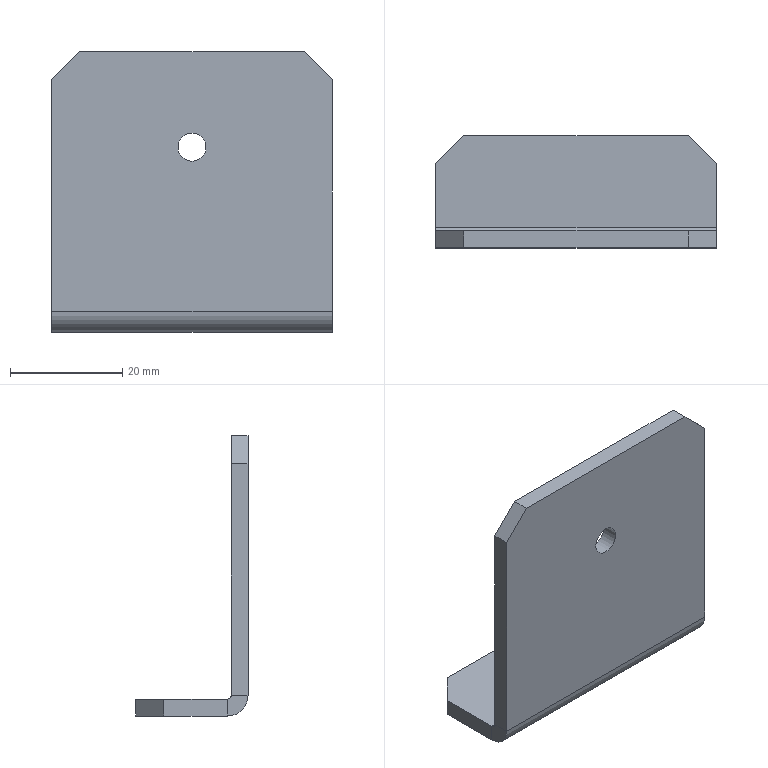Part | NX | 1 solid | 19 faces | box 50 x 20 x 50 mm | volume 9696 mm3 | plane 16 | cylinder 3 | commonest cylinder face diameters 1.5 x1 5 x1 7.5 x1
STEP:
#1=CARTESIAN_POINT('',(25.,0.,3.75));
#2=VERTEX_POINT('',#1);
#3=CARTESIAN_POINT('',(25.,3.,3.75));
#4=VERTEX_POINT('',#3);
#5=CARTESIAN_POINT('',(25.,0.,3.75));
#6=DIRECTION('',(0.,1.,0.));
#7=VECTOR('',#6,1000.);
#8=LINE('',#5,#7);
#9=EDGE_CURVE('',#2,#4,#8,.T.);
#10=ORIENTED_EDGE('',*,*,#9,.F.);
#11=CARTESIAN_POINT('',(25.,3.75,0.));
#12=VERTEX_POINT('',#11);
#13=CARTESIAN_POINT('',(25.,3.75,3.75));
#14=DIRECTION('',(1.,0.,0.));
#15=DIRECTION('',(0.,0.,-1.));
#16=AXIS2_PLACEMENT_3D('',#13,#14,#15);
#17=CIRCLE('',#16,3.75);
#18=EDGE_CURVE('',#12,#2,#17,.F.);
#19=ORIENTED_EDGE('',*,*,#18,.F.);
#20=CARTESIAN_POINT('',(25.,3.75,3.));
#21=VERTEX_POINT('',#20);
#22=CARTESIAN_POINT('',(25.,3.75,3.));
#23=DIRECTION('',(0.,0.,-1.));
#24=VECTOR('',#23,1000.);
#25=LINE('',#22,#24);
#26=EDGE_CURVE('',#21,#12,#25,.T.);
#27=ORIENTED_EDGE('',*,*,#26,.F.);
#28=CARTESIAN_POINT('',(25.,3.75,3.75));
#29=DIRECTION('',(1.,0.,0.));
#30=DIRECTION('',(0.,0.,-1.));
#31=AXIS2_PLACEMENT_3D('',#28,#29,#30);
#32=CIRCLE('',#31,0.75);
#33=EDGE_CURVE('',#21,#4,#32,.F.);
#34=ORIENTED_EDGE('',*,*,#33,.T.);
#35=EDGE_LOOP('',(#10,#19,#27,#34));
#36=FACE_BOUND('',#35,.T.);
#37=CARTESIAN_POINT('',(25.,0.,3.75));
#38=DIRECTION('',(1.,0.,0.));
#39=DIRECTION('',(0.,0.,-1.));
#40=AXIS2_PLACEMENT_3D('',#37,#38,#39);
#41=PLANE('',#40);
#42=ADVANCED_FACE('',(#36),#41,.T.);
#43=CARTESIAN_POINT('',(25.,3.,45.));
#44=VERTEX_POINT('',#43);
#45=CARTESIAN_POINT('',(25.,3.,0.));
#46=DIRECTION('',(0.,0.,1.));
#47=VECTOR('',#46,1000.);
#48=LINE('',#45,#47);
#49=EDGE_CURVE('',#4,#44,#48,.T.);
#50=ORIENTED_EDGE('',*,*,#49,.T.);
#51=CARTESIAN_POINT('',(25.,0.,45.));
#52=VERTEX_POINT('',#51);
#53=CARTESIAN_POINT('',(25.,3.75,45.));
#54=DIRECTION('',(0.,-1.,0.));
#55=VECTOR('',#54,1000.);
#56=LINE('',#53,#55);
#57=EDGE_CURVE('',#44,#52,#56,.T.);
#58=ORIENTED_EDGE('',*,*,#57,.T.);
#59=CARTESIAN_POINT('',(25.,0.,0.));
#60=DIRECTION('',(0.,0.,1.));
#61=VECTOR('',#60,1000.);
#62=LINE('',#59,#61);
#63=EDGE_CURVE('',#2,#52,#62,.T.);
#64=ORIENTED_EDGE('',*,*,#63,.F.);
#65=ORIENTED_EDGE('',*,*,#9,.T.);
#66=EDGE_LOOP('',(#50,#58,#64,#65));
#67=FACE_BOUND('',#66,.T.);
#68=CARTESIAN_POINT('',(25.,3.75,3.));
#69=DIRECTION('',(1.,0.,0.));
#70=DIRECTION('',(0.,0.,-1.));
#71=AXIS2_PLACEMENT_3D('',#68,#69,#70);
#72=PLANE('',#71);
#73=ADVANCED_FACE('',(#67),#72,.T.);
#74=CARTESIAN_POINT('',(-25.,3.75,0.));
#75=VERTEX_POINT('',#74);
#76=CARTESIAN_POINT('',(-25.,3.75,3.));
#77=VERTEX_POINT('',#76);
#78=CARTESIAN_POINT('',(-25.,3.75,0.));
#79=DIRECTION('',(0.,0.,1.));
#80=VECTOR('',#79,1000.);
#81=LINE('',#78,#80);
#82=EDGE_CURVE('',#75,#77,#81,.T.);
#83=ORIENTED_EDGE('',*,*,#82,.F.);
#84=CARTESIAN_POINT('',(-25.,0.,3.75));
#85=VERTEX_POINT('',#84);
#86=CARTESIAN_POINT('',(-25.,3.75,3.75));
#87=DIRECTION('',(1.,0.,0.));
#88=DIRECTION('',(0.,0.,-1.));
#89=AXIS2_PLACEMENT_3D('',#86,#87,#88);
#90=CIRCLE('',#89,3.75);
#91=EDGE_CURVE('',#75,#85,#90,.F.);
#92=ORIENTED_EDGE('',*,*,#91,.T.);
#93=CARTESIAN_POINT('',(-25.,3.,3.75));
#94=VERTEX_POINT('',#93);
#95=CARTESIAN_POINT('',(-25.,3.,3.75));
#96=DIRECTION('',(0.,-1.,0.));
#97=VECTOR('',#96,1000.);
#98=LINE('',#95,#97);
#99=EDGE_CURVE('',#94,#85,#98,.T.);
#100=ORIENTED_EDGE('',*,*,#99,.F.);
#101=CARTESIAN_POINT('',(-25.,3.75,3.75));
#102=DIRECTION('',(1.,0.,0.));
#103=DIRECTION('',(0.,0.,-1.));
#104=AXIS2_PLACEMENT_3D('',#101,#102,#103);
#105=CIRCLE('',#104,0.75);
#106=EDGE_CURVE('',#77,#94,#105,.F.);
#107=ORIENTED_EDGE('',*,*,#106,.F.);
#108=EDGE_LOOP('',(#83,#92,#100,#107));
#109=FACE_BOUND('',#108,.T.);
#110=CARTESIAN_POINT('',(-25.,3.75,0.));
#111=DIRECTION('',(-1.,0.,0.));
#112=DIRECTION('',(0.,0.,1.));
#113=AXIS2_PLACEMENT_3D('',#110,#111,#112);
#114=PLANE('',#113);
#115=ADVANCED_FACE('',(#109),#114,.T.);
#116=CARTESIAN_POINT('',(-25.,15.,3.));
#117=VERTEX_POINT('',#116);
#118=CARTESIAN_POINT('',(-25.,20.,3.));
#119=DIRECTION('',(0.,-1.,0.));
#120=VECTOR('',#119,1000.);
#121=LINE('',#118,#120);
#122=EDGE_CURVE('',#117,#77,#121,.T.);
#123=ORIENTED_EDGE('',*,*,#122,.F.);
#124=CARTESIAN_POINT('',(-25.,15.,0.));
#125=VERTEX_POINT('',#124);
#126=CARTESIAN_POINT('',(-25.,15.,3.75));
#127=DIRECTION('',(0.,0.,-1.));
#128=VECTOR('',#127,1000.);
#129=LINE('',#126,#128);
#130=EDGE_CURVE('',#117,#125,#129,.T.);
#131=ORIENTED_EDGE('',*,*,#130,.T.);
#132=CARTESIAN_POINT('',(-25.,20.,0.));
#133=DIRECTION('',(0.,-1.,0.));
#134=VECTOR('',#133,1000.);
#135=LINE('',#132,#134);
#136=EDGE_CURVE('',#125,#75,#135,.T.);
#137=ORIENTED_EDGE('',*,*,#136,.T.);
#138=ORIENTED_EDGE('',*,*,#82,.T.);
#139=EDGE_LOOP('',(#123,#131,#137,#138));
#140=FACE_BOUND('',#139,.T.);
#141=CARTESIAN_POINT('',(-25.,3.,3.75));
#142=DIRECTION('',(-1.,0.,0.));
#143=DIRECTION('',(0.,0.,1.));
#144=AXIS2_PLACEMENT_3D('',#141,#142,#143);
#145=PLANE('',#144);
#146=ADVANCED_FACE('',(#140),#145,.T.);
#147=CARTESIAN_POINT('',(0.,3.,30.5));
#148=VERTEX_POINT('',#147);
#149=CARTESIAN_POINT('',(0.,3.,33.));
#150=DIRECTION('',(0.,-1.,0.));
#151=DIRECTION('',(0.,0.,-1.));
#152=AXIS2_PLACEMENT_3D('',#149,#150,#151);
#153=CIRCLE('',#152,2.5);
#154=EDGE_CURVE('',#148,#148,#153,.T.);
#155=ORIENTED_EDGE('',*,*,#154,.T.);
#156=EDGE_LOOP('',(#155));
#157=FACE_BOUND('',#156,.T.);
#158=CARTESIAN_POINT('',(20.,3.,50.));
#159=VERTEX_POINT('',#158);
#160=CARTESIAN_POINT('',(-20.,3.,50.));
#161=VERTEX_POINT('',#160);
#162=CARTESIAN_POINT('',(25.,3.,50.));
#163=DIRECTION('',(-1.,0.,0.));
#164=VECTOR('',#163,1000.);
#165=LINE('',#162,#164);
#166=EDGE_CURVE('',#159,#161,#165,.T.);
#167=ORIENTED_EDGE('',*,*,#166,.F.);
#168=CARTESIAN_POINT('',(20.,3.,50.));
#169=DIRECTION('',(-0.7071,0.,0.7071));
#170=VECTOR('',#169,1000.);
#171=LINE('',#168,#170);
#172=EDGE_CURVE('',#159,#44,#171,.F.);
#173=ORIENTED_EDGE('',*,*,#172,.T.);
#174=ORIENTED_EDGE('',*,*,#49,.F.);
#175=CARTESIAN_POINT('',(25.,3.,3.75));
#176=DIRECTION('',(-1.,0.,0.));
#177=VECTOR('',#176,1000.);
#178=LINE('',#175,#177);
#179=EDGE_CURVE('',#4,#94,#178,.T.);
#180=ORIENTED_EDGE('',*,*,#179,.T.);
#181=CARTESIAN_POINT('',(-25.,3.,45.));
#182=VERTEX_POINT('',#181);
#183=CARTESIAN_POINT('',(-25.,3.,0.));
#184=DIRECTION('',(0.,0.,1.));
#185=VECTOR('',#184,1000.);
#186=LINE('',#183,#185);
#187=EDGE_CURVE('',#94,#182,#186,.T.);
#188=ORIENTED_EDGE('',*,*,#187,.T.);
#189=CARTESIAN_POINT('',(-25.,3.,45.));
#190=DIRECTION('',(0.7071,0.,0.7071));
#191=VECTOR('',#190,1000.);
#192=LINE('',#189,#191);
#193=EDGE_CURVE('',#182,#161,#192,.T.);
#194=ORIENTED_EDGE('',*,*,#193,.T.);
#195=EDGE_LOOP('',(#167,#173,#174,#180,#188,#194));
#196=FACE_BOUND('',#195,.T.);
#197=CARTESIAN_POINT('',(25.,3.,0.));
#198=DIRECTION('',(0.,-1.,0.));
#199=DIRECTION('',(0.,0.,-1.));
#200=AXIS2_PLACEMENT_3D('',#197,#198,#199);
#201=PLANE('',#200);
#202=ADVANCED_FACE('',(#157,#196),#201,.F.);
#203=CARTESIAN_POINT('',(20.,0.,50.));
#204=VERTEX_POINT('',#203);
#205=CARTESIAN_POINT('',(-20.,0.,50.));
#206=VERTEX_POINT('',#205);
#207=CARTESIAN_POINT('',(25.,0.,50.));
#208=DIRECTION('',(-1.,0.,0.));
#209=VECTOR('',#208,1000.);
#210=LINE('',#207,#209);
#211=EDGE_CURVE('',#204,#206,#210,.T.);
#212=ORIENTED_EDGE('',*,*,#211,.F.);
#213=CARTESIAN_POINT('',(20.,0.,50.));
#214=DIRECTION('',(0.,1.,0.));
#215=VECTOR('',#214,1000.);
#216=LINE('',#213,#215);
#217=EDGE_CURVE('',#204,#159,#216,.T.);
#218=ORIENTED_EDGE('',*,*,#217,.T.);
#219=ORIENTED_EDGE('',*,*,#166,.T.);
#220=CARTESIAN_POINT('',(-20.,0.,50.));
#221=DIRECTION('',(0.,-1.,0.));
#222=VECTOR('',#221,1000.);
#223=LINE('',#220,#222);
#224=EDGE_CURVE('',#161,#206,#223,.T.);
#225=ORIENTED_EDGE('',*,*,#224,.T.);
#226=EDGE_LOOP('',(#212,#218,#219,#225));
#227=FACE_BOUND('',#226,.T.);
#228=CARTESIAN_POINT('',(25.,0.,50.));
#229=DIRECTION('',(0.,0.,1.));
#230=DIRECTION('',(1.,0.,0.));
#231=AXIS2_PLACEMENT_3D('',#228,#229,#230);
#232=PLANE('',#231);
#233=ADVANCED_FACE('',(#227),#232,.T.);
#234=CARTESIAN_POINT('',(0.,0.,30.5));
#235=VERTEX_POINT('',#234);
#236=CARTESIAN_POINT('',(0.,0.,33.));
#237=DIRECTION('',(0.,-1.,0.));
#238=DIRECTION('',(0.,0.,-1.));
#239=AXIS2_PLACEMENT_3D('',#236,#237,#238);
#240=CIRCLE('',#239,2.5);
#241=EDGE_CURVE('',#235,#235,#240,.T.);
#242=ORIENTED_EDGE('',*,*,#241,.F.);
#243=EDGE_LOOP('',(#242));
#244=FACE_BOUND('',#243,.T.);
#245=ORIENTED_EDGE('',*,*,#63,.T.);
#246=CARTESIAN_POINT('',(47.5,0.,22.5));
#247=DIRECTION('',(0.7071,0.,-0.7071));
#248=VECTOR('',#247,1000.);
#249=LINE('',#246,#248);
#250=EDGE_CURVE('',#52,#204,#249,.F.);
#251=ORIENTED_EDGE('',*,*,#250,.T.);
#252=ORIENTED_EDGE('',*,*,#211,.T.);
#253=CARTESIAN_POINT('',(-25.,0.,45.));
#254=VERTEX_POINT('',#253);
#255=CARTESIAN_POINT('',(-22.5,0.,47.5));
#256=DIRECTION('',(-0.7071,0.,-0.7071));
#257=VECTOR('',#256,1000.);
#258=LINE('',#255,#257);
#259=EDGE_CURVE('',#206,#254,#258,.T.);
#260=ORIENTED_EDGE('',*,*,#259,.T.);
#261=CARTESIAN_POINT('',(-25.,0.,0.));
#262=DIRECTION('',(0.,0.,1.));
#263=VECTOR('',#262,1000.);
#264=LINE('',#261,#263);
#265=EDGE_CURVE('',#85,#254,#264,.T.);
#266=ORIENTED_EDGE('',*,*,#265,.F.);
#267=CARTESIAN_POINT('',(25.,0.,3.75));
#268=DIRECTION('',(-1.,0.,0.));
#269=VECTOR('',#268,1000.);
#270=LINE('',#267,#269);
#271=EDGE_CURVE('',#2,#85,#270,.T.);
#272=ORIENTED_EDGE('',*,*,#271,.F.);
#273=EDGE_LOOP('',(#245,#251,#252,#260,#266,#272));
#274=FACE_BOUND('',#273,.T.);
#275=CARTESIAN_POINT('',(25.,0.,0.));
#276=DIRECTION('',(0.,-1.,0.));
#277=DIRECTION('',(0.,0.,-1.));
#278=AXIS2_PLACEMENT_3D('',#275,#276,#277);
#279=PLANE('',#278);
#280=ADVANCED_FACE('',(#244,#274),#279,.T.);
#281=ORIENTED_EDGE('',*,*,#91,.F.);
#282=CARTESIAN_POINT('',(25.,3.75,0.));
#283=DIRECTION('',(-1.,0.,0.));
#284=VECTOR('',#283,1000.);
#285=LINE('',#282,#284);
#286=EDGE_CURVE('',#12,#75,#285,.T.);
#287=ORIENTED_EDGE('',*,*,#286,.F.);
#288=ORIENTED_EDGE('',*,*,#18,.T.);
#289=ORIENTED_EDGE('',*,*,#271,.T.);
#290=EDGE_LOOP('',(#281,#287,#288,#289));
#291=FACE_BOUND('',#290,.T.);
#292=CARTESIAN_POINT('',(25.,3.75,3.75));
#293=DIRECTION('',(-1.,0.,0.));
#294=DIRECTION('',(0.,0.,1.));
#295=AXIS2_PLACEMENT_3D('',#292,#293,#294);
#296=CYLINDRICAL_SURFACE('',#295,3.75);
#297=ADVANCED_FACE('',(#291),#296,.T.);
#298=CARTESIAN_POINT('',(20.,20.,0.));
#299=VERTEX_POINT('',#298);
#300=CARTESIAN_POINT('',(-20.,20.,0.));
#301=VERTEX_POINT('',#300);
#302=CARTESIAN_POINT('',(25.,20.,0.));
#303=DIRECTION('',(-1.,0.,0.));
#304=VECTOR('',#303,1000.);
#305=LINE('',#302,#304);
#306=EDGE_CURVE('',#299,#301,#305,.T.);
#307=ORIENTED_EDGE('',*,*,#306,.F.);
#308=CARTESIAN_POINT('',(25.,15.,0.));
#309=VERTEX_POINT('',#308);
#310=CARTESIAN_POINT('',(22.5,17.5,0.));
#311=DIRECTION('',(-0.7071,0.7071,0.));
#312=VECTOR('',#311,1000.);
#313=LINE('',#310,#312);
#314=EDGE_CURVE('',#299,#309,#313,.F.);
#315=ORIENTED_EDGE('',*,*,#314,.T.);
#316=CARTESIAN_POINT('',(25.,20.,0.));
#317=DIRECTION('',(0.,-1.,0.));
#318=VECTOR('',#317,1000.);
#319=LINE('',#316,#318);
#320=EDGE_CURVE('',#309,#12,#319,.T.);
#321=ORIENTED_EDGE('',*,*,#320,.T.);
#322=ORIENTED_EDGE('',*,*,#286,.T.);
#323=ORIENTED_EDGE('',*,*,#136,.F.);
#324=CARTESIAN_POINT('',(2.5,42.5,0.));
#325=DIRECTION('',(-0.7071,-0.7071,0.));
#326=VECTOR('',#325,1000.);
#327=LINE('',#324,#326);
#328=EDGE_CURVE('',#125,#301,#327,.F.);
#329=ORIENTED_EDGE('',*,*,#328,.T.);
#330=EDGE_LOOP('',(#307,#315,#321,#322,#323,#329));
#331=FACE_BOUND('',#330,.T.);
#332=CARTESIAN_POINT('',(25.,20.,0.));
#333=DIRECTION('',(0.,0.,-1.));
#334=DIRECTION('',(0.,1.,0.));
#335=AXIS2_PLACEMENT_3D('',#332,#333,#334);
#336=PLANE('',#335);
#337=ADVANCED_FACE('',(#331),#336,.T.);
#338=CARTESIAN_POINT('',(20.,20.,3.));
#339=VERTEX_POINT('',#338);
#340=CARTESIAN_POINT('',(-20.,20.,3.));
#341=VERTEX_POINT('',#340);
#342=CARTESIAN_POINT('',(25.,20.,3.));
#343=DIRECTION('',(-1.,0.,0.));
#344=VECTOR('',#343,1000.);
#345=LINE('',#342,#344);
#346=EDGE_CURVE('',#339,#341,#345,.T.);
#347=ORIENTED_EDGE('',*,*,#346,.F.);
#348=CARTESIAN_POINT('',(20.,20.,3.));
#349=DIRECTION('',(0.,0.,-1.));
#350=VECTOR('',#349,1000.);
#351=LINE('',#348,#350);
#352=EDGE_CURVE('',#339,#299,#351,.T.);
#353=ORIENTED_EDGE('',*,*,#352,.T.);
#354=ORIENTED_EDGE('',*,*,#306,.T.);
#355=CARTESIAN_POINT('',(-20.,20.,3.));
#356=DIRECTION('',(0.,0.,1.));
#357=VECTOR('',#356,1000.);
#358=LINE('',#355,#357);
#359=EDGE_CURVE('',#301,#341,#358,.T.);
#360=ORIENTED_EDGE('',*,*,#359,.T.);
#361=EDGE_LOOP('',(#347,#353,#354,#360));
#362=FACE_BOUND('',#361,.T.);
#363=CARTESIAN_POINT('',(25.,20.,3.));
#364=DIRECTION('',(0.,1.,0.));
#365=DIRECTION('',(0.,0.,1.));
#366=AXIS2_PLACEMENT_3D('',#363,#364,#365);
#367=PLANE('',#366);
#368=ADVANCED_FACE('',(#362),#367,.T.);
#369=CARTESIAN_POINT('',(25.,15.,3.));
#370=VERTEX_POINT('',#369);
#371=CARTESIAN_POINT('',(25.,20.,3.));
#372=DIRECTION('',(0.,-1.,0.));
#373=VECTOR('',#372,1000.);
#374=LINE('',#371,#373);
#375=EDGE_CURVE('',#370,#21,#374,.T.);
#376=ORIENTED_EDGE('',*,*,#375,.F.);
#377=CARTESIAN_POINT('',(20.,20.,3.));
#378=DIRECTION('',(0.7071,-0.7071,0.));
#379=VECTOR('',#378,1000.);
#380=LINE('',#377,#379);
#381=EDGE_CURVE('',#370,#339,#380,.F.);
#382=ORIENTED_EDGE('',*,*,#381,.T.);
#383=ORIENTED_EDGE('',*,*,#346,.T.);
#384=CARTESIAN_POINT('',(-25.,15.,3.));
#385=DIRECTION('',(0.7071,0.7071,0.));
#386=VECTOR('',#385,1000.);
#387=LINE('',#384,#386);
#388=EDGE_CURVE('',#341,#117,#387,.F.);
#389=ORIENTED_EDGE('',*,*,#388,.T.);
#390=ORIENTED_EDGE('',*,*,#122,.T.);
#391=CARTESIAN_POINT('',(25.,3.75,3.));
#392=DIRECTION('',(-1.,0.,0.));
#393=VECTOR('',#392,1000.);
#394=LINE('',#391,#393);
#395=EDGE_CURVE('',#21,#77,#394,.T.);
#396=ORIENTED_EDGE('',*,*,#395,.F.);
#397=EDGE_LOOP('',(#376,#382,#383,#389,#390,#396));
#398=FACE_BOUND('',#397,.T.);
#399=CARTESIAN_POINT('',(25.,20.,3.));
#400=DIRECTION('',(0.,0.,-1.));
#401=DIRECTION('',(0.,1.,0.));
#402=AXIS2_PLACEMENT_3D('',#399,#400,#401);
#403=PLANE('',#402);
#404=ADVANCED_FACE('',(#398),#403,.F.);
#405=ORIENTED_EDGE('',*,*,#106,.T.);
#406=ORIENTED_EDGE('',*,*,#179,.F.);
#407=ORIENTED_EDGE('',*,*,#33,.F.);
#408=ORIENTED_EDGE('',*,*,#395,.T.);
#409=EDGE_LOOP('',(#405,#406,#407,#408));
#410=FACE_BOUND('',#409,.T.);
#411=CARTESIAN_POINT('',(25.,3.75,3.75));
#412=DIRECTION('',(-1.,0.,0.));
#413=DIRECTION('',(0.,0.,1.));
#414=AXIS2_PLACEMENT_3D('',#411,#412,#413);
#415=CYLINDRICAL_SURFACE('',#414,0.75);
#416=ADVANCED_FACE('',(#410),#415,.F.);
#417=ORIENTED_EDGE('',*,*,#320,.F.);
#418=CARTESIAN_POINT('',(25.,15.,3.75));
#419=DIRECTION('',(0.,0.,1.));
#420=VECTOR('',#419,1000.);
#421=LINE('',#418,#420);
#422=EDGE_CURVE('',#309,#370,#421,.T.);
#423=ORIENTED_EDGE('',*,*,#422,.T.);
#424=ORIENTED_EDGE('',*,*,#375,.T.);
#425=ORIENTED_EDGE('',*,*,#26,.T.);
#426=EDGE_LOOP('',(#417,#423,#424,#425));
#427=FACE_BOUND('',#426,.T.);
#428=CARTESIAN_POINT('',(25.,3.75,3.75));
#429=DIRECTION('',(1.,0.,0.));
#430=DIRECTION('',(0.,0.,-1.));
#431=AXIS2_PLACEMENT_3D('',#428,#429,#430);
#432=PLANE('',#431);
#433=ADVANCED_FACE('',(#427),#432,.T.);
#434=ORIENTED_EDGE('',*,*,#265,.T.);
#435=CARTESIAN_POINT('',(-25.,3.,45.));
#436=DIRECTION('',(0.,1.,0.));
#437=VECTOR('',#436,1000.);
#438=LINE('',#435,#437);
#439=EDGE_CURVE('',#254,#182,#438,.T.);
#440=ORIENTED_EDGE('',*,*,#439,.T.);
#441=ORIENTED_EDGE('',*,*,#187,.F.);
#442=ORIENTED_EDGE('',*,*,#99,.T.);
#443=EDGE_LOOP('',(#434,#440,#441,#442));
#444=FACE_BOUND('',#443,.T.);
#445=CARTESIAN_POINT('',(-25.,3.75,3.75));
#446=DIRECTION('',(1.,0.,0.));
#447=DIRECTION('',(0.,0.,-1.));
#448=AXIS2_PLACEMENT_3D('',#445,#446,#447);
#449=PLANE('',#448);
#450=ADVANCED_FACE('',(#444),#449,.F.);
#451=ORIENTED_EDGE('',*,*,#241,.T.);
#452=EDGE_LOOP('',(#451));
#453=FACE_BOUND('',#452,.T.);
#454=ORIENTED_EDGE('',*,*,#154,.F.);
#455=EDGE_LOOP('',(#454));
#456=FACE_BOUND('',#455,.T.);
#457=CARTESIAN_POINT('',(0.,0.,33.));
#458=DIRECTION('',(0.,-1.,0.));
#459=DIRECTION('',(0.,0.,-1.));
#460=AXIS2_PLACEMENT_3D('',#457,#458,#459);
#461=CYLINDRICAL_SURFACE('',#460,2.5);
#462=ADVANCED_FACE('',(#453,#456),#461,.F.);
#463=ORIENTED_EDGE('',*,*,#381,.F.);
#464=ORIENTED_EDGE('',*,*,#422,.F.);
#465=ORIENTED_EDGE('',*,*,#314,.F.);
#466=ORIENTED_EDGE('',*,*,#352,.F.);
#467=EDGE_LOOP('',(#463,#464,#465,#466));
#468=FACE_BOUND('',#467,.T.);
#469=CARTESIAN_POINT('',(20.,20.,3.));
#470=DIRECTION('',(-0.7071,-0.7071,0.));
#471=DIRECTION('',(0.,0.,-1.));
#472=AXIS2_PLACEMENT_3D('',#469,#470,#471);
#473=PLANE('',#472);
#474=ADVANCED_FACE('',(#468),#473,.F.);
#475=ORIENTED_EDGE('',*,*,#388,.F.);
#476=ORIENTED_EDGE('',*,*,#359,.F.);
#477=ORIENTED_EDGE('',*,*,#328,.F.);
#478=ORIENTED_EDGE('',*,*,#130,.F.);
#479=EDGE_LOOP('',(#475,#476,#477,#478));
#480=FACE_BOUND('',#479,.T.);
#481=CARTESIAN_POINT('',(-25.,15.,3.75));
#482=DIRECTION('',(0.7071,-0.7071,0.));
#483=DIRECTION('',(0.,0.,-1.));
#484=AXIS2_PLACEMENT_3D('',#481,#482,#483);
#485=PLANE('',#484);
#486=ADVANCED_FACE('',(#480),#485,.F.);
#487=ORIENTED_EDGE('',*,*,#250,.F.);
#488=ORIENTED_EDGE('',*,*,#57,.F.);
#489=ORIENTED_EDGE('',*,*,#172,.F.);
#490=ORIENTED_EDGE('',*,*,#217,.F.);
#491=EDGE_LOOP('',(#487,#488,#489,#490));
#492=FACE_BOUND('',#491,.T.);
#493=CARTESIAN_POINT('',(20.,0.,50.));
#494=DIRECTION('',(-0.7071,0.,-0.7071));
#495=DIRECTION('',(0.,1.,0.));
#496=AXIS2_PLACEMENT_3D('',#493,#494,#495);
#497=PLANE('',#496);
#498=ADVANCED_FACE('',(#492),#497,.F.);
#499=ORIENTED_EDGE('',*,*,#259,.F.);
#500=ORIENTED_EDGE('',*,*,#224,.F.);
#501=ORIENTED_EDGE('',*,*,#193,.F.);
#502=ORIENTED_EDGE('',*,*,#439,.F.);
#503=EDGE_LOOP('',(#499,#500,#501,#502));
#504=FACE_BOUND('',#503,.T.);
#505=CARTESIAN_POINT('',(-25.,3.75,45.));
#506=DIRECTION('',(-0.7071,0.,0.7071));
#507=DIRECTION('',(0.,-1.,0.));
#508=AXIS2_PLACEMENT_3D('',#505,#506,#507);
#509=PLANE('',#508);
#510=ADVANCED_FACE('',(#504),#509,.T.);
#511=CLOSED_SHELL('',(#42,#73,#115,#146,#202,#233,#280,#297,#337,#368,#404,#416,#433,#450,#462,#474,#486,#498,#510));
#512=MANIFOLD_SOLID_BREP('',#511);
#513=(LENGTH_UNIT()NAMED_UNIT(*)SI_UNIT(.MILLI.,.METRE.));
#514=UNCERTAINTY_MEASURE_WITH_UNIT(LENGTH_MEASURE(0.00001),#513,'','');
#515=(NAMED_UNIT(*)PLANE_ANGLE_UNIT()SI_UNIT($,.RADIAN.));
#516=(NAMED_UNIT(*)SI_UNIT($,.STERADIAN.)SOLID_ANGLE_UNIT());
#517=(GEOMETRIC_REPRESENTATION_CONTEXT(3)GLOBAL_UNCERTAINTY_ASSIGNED_CONTEXT((#514))GLOBAL_UNIT_ASSIGNED_CONTEXT((#513,#515,#516))REPRESENTATION_CONTEXT('',''));
#518=ADVANCED_BREP_SHAPE_REPRESENTATION('',(#512),#517);